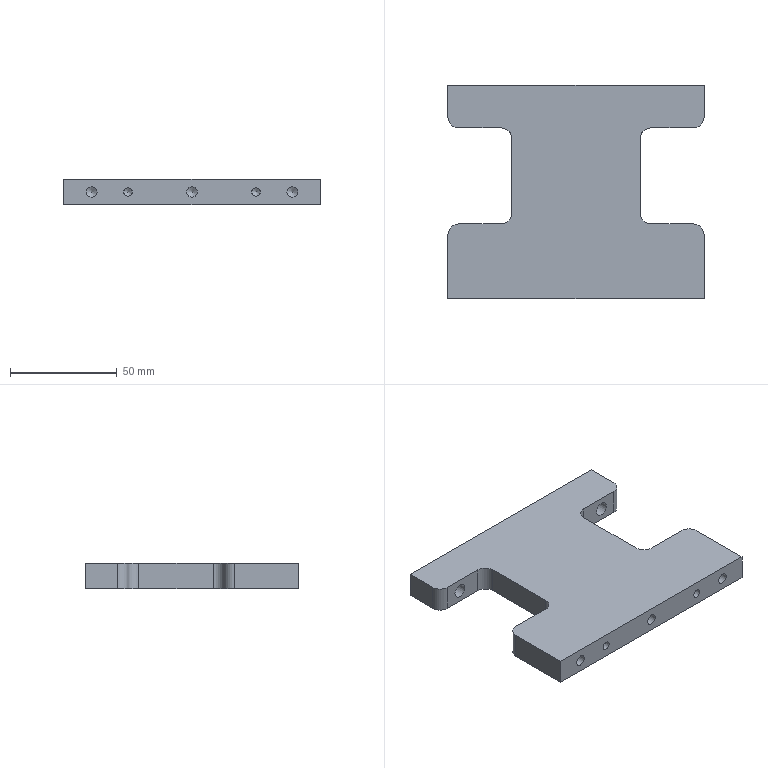Part | STEP file | SynoNew-0304-024 | 1 solid | 34 faces | box 120 x 100 x 12 mm | volume 109561 mm3 | cylinder 15 | plane 14 | cone 5 | commonest cylinder face diameters 10 x8 5 x3 4 x2 6.5 x2
STEP:
#1=CARTESIAN_POINT('',(32.,-42.,6.));
#2=VERTEX_POINT('',#1);
#3=CARTESIAN_POINT('',(28.,-42.,6.));
#4=VERTEX_POINT('',#3);
#5=CARTESIAN_POINT('',(30.,-42.,6.));
#6=DIRECTION('',(0.,-1.,0.));
#7=DIRECTION('',(1.,0.,0.));
#8=AXIS2_PLACEMENT_3D('',#5,#6,#7);
#9=CIRCLE('',#8,2.);
#10=EDGE_CURVE('',#2,#4,#9,.T.);
#11=ORIENTED_EDGE('',*,*,#10,.T.);
#12=CARTESIAN_POINT('',(30.,-40.798,6.));
#13=VERTEX_POINT('',#12);
#14=CARTESIAN_POINT('',(29.,-41.399,6.));
#15=DIRECTION('',(0.8572,0.515,0.));
#16=VECTOR('',#15,1.);
#17=LINE('',#14,#16);
#18=EDGE_CURVE('',#4,#13,#17,.T.);
#19=ORIENTED_EDGE('',*,*,#18,.T.);
#20=ORIENTED_EDGE('',*,*,#18,.F.);
#21=CARTESIAN_POINT('',(30.,-42.,6.));
#22=DIRECTION('',(0.,-1.,0.));
#23=DIRECTION('',(1.,0.,0.));
#24=AXIS2_PLACEMENT_3D('',#21,#22,#23);
#25=CIRCLE('',#24,2.);
#26=EDGE_CURVE('',#4,#2,#25,.T.);
#27=ORIENTED_EDGE('',*,*,#26,.T.);
#28=EDGE_LOOP('',(#11,#19,#20,#27));
#29=FACE_OUTER_BOUND('',#28,.T.);
#30=CARTESIAN_POINT('',(30.,-41.399,6.));
#31=DIRECTION('',(0.,-1.,0.));
#32=DIRECTION('',(1.,0.,0.));
#33=AXIS2_PLACEMENT_3D('',#30,#31,#32);
#34=CONICAL_SURFACE('',#33,1.,1.03);
#35=ADVANCED_FACE('',(#29),#34,.F.);
#36=CARTESIAN_POINT('',(32.,-50.,6.));
#37=VERTEX_POINT('',#36);
#38=CARTESIAN_POINT('',(28.,-50.,6.));
#39=VERTEX_POINT('',#38);
#40=CARTESIAN_POINT('',(30.,-50.,6.));
#41=DIRECTION('',(0.,1.,0.));
#42=DIRECTION('',(1.,0.,0.));
#43=AXIS2_PLACEMENT_3D('',#40,#41,#42);
#44=CIRCLE('',#43,2.);
#45=EDGE_CURVE('',#37,#39,#44,.T.);
#46=ORIENTED_EDGE('',*,*,#45,.F.);
#47=CARTESIAN_POINT('',(30.,-50.,6.));
#48=DIRECTION('',(0.,1.,0.));
#49=DIRECTION('',(1.,0.,0.));
#50=AXIS2_PLACEMENT_3D('',#47,#48,#49);
#51=CIRCLE('',#50,2.);
#52=EDGE_CURVE('',#39,#37,#51,.T.);
#53=ORIENTED_EDGE('',*,*,#52,.F.);
#54=CARTESIAN_POINT('',(28.,-46.,6.));
#55=DIRECTION('',(0.,1.,0.));
#56=VECTOR('',#55,2.);
#57=LINE('',#54,#56);
#58=EDGE_CURVE('',#39,#4,#57,.T.);
#59=ORIENTED_EDGE('',*,*,#58,.T.);
#60=ORIENTED_EDGE('',*,*,#10,.F.);
#61=ORIENTED_EDGE('',*,*,#26,.F.);
#62=ORIENTED_EDGE('',*,*,#58,.F.);
#63=EDGE_LOOP('',(#46,#53,#59,#60,#61,#62));
#64=FACE_OUTER_BOUND('',#63,.T.);
#65=CARTESIAN_POINT('',(30.,-46.,6.));
#66=DIRECTION('',(0.,-1.,0.));
#67=DIRECTION('',(1.,0.,0.));
#68=AXIS2_PLACEMENT_3D('',#65,#66,#67);
#69=CYLINDRICAL_SURFACE('',#68,2.);
#70=ADVANCED_FACE('',(#64),#69,.F.);
#71=CARTESIAN_POINT('',(-28.,-42.,6.));
#72=VERTEX_POINT('',#71);
#73=CARTESIAN_POINT('',(-32.,-42.,6.));
#74=VERTEX_POINT('',#73);
#75=CARTESIAN_POINT('',(-30.,-42.,6.));
#76=DIRECTION('',(0.,-1.,0.));
#77=DIRECTION('',(1.,0.,0.));
#78=AXIS2_PLACEMENT_3D('',#75,#76,#77);
#79=CIRCLE('',#78,2.);
#80=EDGE_CURVE('',#72,#74,#79,.T.);
#81=ORIENTED_EDGE('',*,*,#80,.T.);
#82=CARTESIAN_POINT('',(-30.,-40.798,6.));
#83=VERTEX_POINT('',#82);
#84=CARTESIAN_POINT('',(-31.,-41.399,6.));
#85=DIRECTION('',(0.8572,0.515,0.));
#86=VECTOR('',#85,1.);
#87=LINE('',#84,#86);
#88=EDGE_CURVE('',#74,#83,#87,.T.);
#89=ORIENTED_EDGE('',*,*,#88,.T.);
#90=ORIENTED_EDGE('',*,*,#88,.F.);
#91=CARTESIAN_POINT('',(-30.,-42.,6.));
#92=DIRECTION('',(0.,-1.,0.));
#93=DIRECTION('',(1.,0.,0.));
#94=AXIS2_PLACEMENT_3D('',#91,#92,#93);
#95=CIRCLE('',#94,2.);
#96=EDGE_CURVE('',#74,#72,#95,.T.);
#97=ORIENTED_EDGE('',*,*,#96,.T.);
#98=EDGE_LOOP('',(#81,#89,#90,#97));
#99=FACE_OUTER_BOUND('',#98,.T.);
#100=CARTESIAN_POINT('',(-30.,-41.399,6.));
#101=DIRECTION('',(0.,-1.,0.));
#102=DIRECTION('',(1.,0.,0.));
#103=AXIS2_PLACEMENT_3D('',#100,#101,#102);
#104=CONICAL_SURFACE('',#103,1.,1.03);
#105=ADVANCED_FACE('',(#99),#104,.F.);
#106=CARTESIAN_POINT('',(-28.,-50.,6.));
#107=VERTEX_POINT('',#106);
#108=CARTESIAN_POINT('',(-32.,-50.,6.));
#109=VERTEX_POINT('',#108);
#110=CARTESIAN_POINT('',(-30.,-50.,6.));
#111=DIRECTION('',(0.,1.,0.));
#112=DIRECTION('',(1.,0.,0.));
#113=AXIS2_PLACEMENT_3D('',#110,#111,#112);
#114=CIRCLE('',#113,2.);
#115=EDGE_CURVE('',#107,#109,#114,.T.);
#116=ORIENTED_EDGE('',*,*,#115,.F.);
#117=CARTESIAN_POINT('',(-30.,-50.,6.));
#118=DIRECTION('',(0.,1.,0.));
#119=DIRECTION('',(1.,0.,0.));
#120=AXIS2_PLACEMENT_3D('',#117,#118,#119);
#121=CIRCLE('',#120,2.);
#122=EDGE_CURVE('',#109,#107,#121,.T.);
#123=ORIENTED_EDGE('',*,*,#122,.F.);
#124=CARTESIAN_POINT('',(-32.,-46.,6.));
#125=DIRECTION('',(0.,1.,0.));
#126=VECTOR('',#125,2.);
#127=LINE('',#124,#126);
#128=EDGE_CURVE('',#109,#74,#127,.T.);
#129=ORIENTED_EDGE('',*,*,#128,.T.);
#130=ORIENTED_EDGE('',*,*,#80,.F.);
#131=ORIENTED_EDGE('',*,*,#96,.F.);
#132=ORIENTED_EDGE('',*,*,#128,.F.);
#133=EDGE_LOOP('',(#116,#123,#129,#130,#131,#132));
#134=FACE_OUTER_BOUND('',#133,.T.);
#135=CARTESIAN_POINT('',(-30.,-46.,6.));
#136=DIRECTION('',(0.,-1.,0.));
#137=DIRECTION('',(1.,0.,0.));
#138=AXIS2_PLACEMENT_3D('',#135,#136,#137);
#139=CYLINDRICAL_SURFACE('',#138,2.);
#140=ADVANCED_FACE('',(#134),#139,.F.);
#141=CARTESIAN_POINT('',(2.5,-42.,6.));
#142=VERTEX_POINT('',#141);
#143=CARTESIAN_POINT('',(-2.5,-42.,6.));
#144=VERTEX_POINT('',#143);
#145=CARTESIAN_POINT('',(0.,-42.,6.));
#146=DIRECTION('',(0.,-1.,0.));
#147=DIRECTION('',(1.,0.,0.));
#148=AXIS2_PLACEMENT_3D('',#145,#146,#147);
#149=CIRCLE('',#148,2.5);
#150=EDGE_CURVE('',#142,#144,#149,.T.);
#151=ORIENTED_EDGE('',*,*,#150,.T.);
#152=CARTESIAN_POINT('',(0.,-40.498,6.));
#153=VERTEX_POINT('',#152);
#154=CARTESIAN_POINT('',(-1.25,-41.249,6.));
#155=DIRECTION('',(0.8572,0.515,0.));
#156=VECTOR('',#155,1.25);
#157=LINE('',#154,#156);
#158=EDGE_CURVE('',#144,#153,#157,.T.);
#159=ORIENTED_EDGE('',*,*,#158,.T.);
#160=ORIENTED_EDGE('',*,*,#158,.F.);
#161=CARTESIAN_POINT('',(0.,-42.,6.));
#162=DIRECTION('',(0.,-1.,0.));
#163=DIRECTION('',(1.,0.,0.));
#164=AXIS2_PLACEMENT_3D('',#161,#162,#163);
#165=CIRCLE('',#164,2.5);
#166=EDGE_CURVE('',#144,#142,#165,.T.);
#167=ORIENTED_EDGE('',*,*,#166,.T.);
#168=EDGE_LOOP('',(#151,#159,#160,#167));
#169=FACE_OUTER_BOUND('',#168,.T.);
#170=CARTESIAN_POINT('',(0.,-41.249,6.));
#171=DIRECTION('',(0.,-1.,0.));
#172=DIRECTION('',(1.,0.,0.));
#173=AXIS2_PLACEMENT_3D('',#170,#171,#172);
#174=CONICAL_SURFACE('',#173,1.25,1.03);
#175=ADVANCED_FACE('',(#169),#174,.F.);
#176=CARTESIAN_POINT('',(2.5,-50.,6.));
#177=VERTEX_POINT('',#176);
#178=CARTESIAN_POINT('',(-2.5,-50.,6.));
#179=VERTEX_POINT('',#178);
#180=CARTESIAN_POINT('',(0.,-50.,6.));
#181=DIRECTION('',(0.,1.,0.));
#182=DIRECTION('',(1.,0.,0.));
#183=AXIS2_PLACEMENT_3D('',#180,#181,#182);
#184=CIRCLE('',#183,2.5);
#185=EDGE_CURVE('',#177,#179,#184,.T.);
#186=ORIENTED_EDGE('',*,*,#185,.F.);
#187=CARTESIAN_POINT('',(0.,-50.,6.));
#188=DIRECTION('',(0.,1.,0.));
#189=DIRECTION('',(1.,0.,0.));
#190=AXIS2_PLACEMENT_3D('',#187,#188,#189);
#191=CIRCLE('',#190,2.5);
#192=EDGE_CURVE('',#179,#177,#191,.T.);
#193=ORIENTED_EDGE('',*,*,#192,.F.);
#194=CARTESIAN_POINT('',(-2.5,-46.,6.));
#195=DIRECTION('',(0.,1.,0.));
#196=VECTOR('',#195,2.5);
#197=LINE('',#194,#196);
#198=EDGE_CURVE('',#179,#144,#197,.T.);
#199=ORIENTED_EDGE('',*,*,#198,.T.);
#200=ORIENTED_EDGE('',*,*,#150,.F.);
#201=ORIENTED_EDGE('',*,*,#166,.F.);
#202=ORIENTED_EDGE('',*,*,#198,.F.);
#203=EDGE_LOOP('',(#186,#193,#199,#200,#201,#202));
#204=FACE_OUTER_BOUND('',#203,.T.);
#205=CARTESIAN_POINT('',(0.,-46.,6.));
#206=DIRECTION('',(0.,-1.,0.));
#207=DIRECTION('',(1.,0.,0.));
#208=AXIS2_PLACEMENT_3D('',#205,#206,#207);
#209=CYLINDRICAL_SURFACE('',#208,2.5);
#210=ADVANCED_FACE('',(#204),#209,.F.);
#211=CARTESIAN_POINT('',(49.5,-42.,6.));
#212=VERTEX_POINT('',#211);
#213=CARTESIAN_POINT('',(44.5,-42.,6.));
#214=VERTEX_POINT('',#213);
#215=CARTESIAN_POINT('',(47.,-42.,6.));
#216=DIRECTION('',(0.,-1.,0.));
#217=DIRECTION('',(1.,0.,0.));
#218=AXIS2_PLACEMENT_3D('',#215,#216,#217);
#219=CIRCLE('',#218,2.5);
#220=EDGE_CURVE('',#212,#214,#219,.T.);
#221=ORIENTED_EDGE('',*,*,#220,.T.);
#222=CARTESIAN_POINT('',(47.,-40.498,6.));
#223=VERTEX_POINT('',#222);
#224=CARTESIAN_POINT('',(45.75,-41.249,6.));
#225=DIRECTION('',(0.8572,0.515,0.));
#226=VECTOR('',#225,1.25);
#227=LINE('',#224,#226);
#228=EDGE_CURVE('',#214,#223,#227,.T.);
#229=ORIENTED_EDGE('',*,*,#228,.T.);
#230=ORIENTED_EDGE('',*,*,#228,.F.);
#231=CARTESIAN_POINT('',(47.,-42.,6.));
#232=DIRECTION('',(0.,-1.,0.));
#233=DIRECTION('',(1.,0.,0.));
#234=AXIS2_PLACEMENT_3D('',#231,#232,#233);
#235=CIRCLE('',#234,2.5);
#236=EDGE_CURVE('',#214,#212,#235,.T.);
#237=ORIENTED_EDGE('',*,*,#236,.T.);
#238=EDGE_LOOP('',(#221,#229,#230,#237));
#239=FACE_OUTER_BOUND('',#238,.T.);
#240=CARTESIAN_POINT('',(47.,-41.249,6.));
#241=DIRECTION('',(0.,-1.,0.));
#242=DIRECTION('',(1.,0.,0.));
#243=AXIS2_PLACEMENT_3D('',#240,#241,#242);
#244=CONICAL_SURFACE('',#243,1.25,1.03);
#245=ADVANCED_FACE('',(#239),#244,.F.);
#246=CARTESIAN_POINT('',(49.5,-50.,6.));
#247=VERTEX_POINT('',#246);
#248=CARTESIAN_POINT('',(44.5,-50.,6.));
#249=VERTEX_POINT('',#248);
#250=CARTESIAN_POINT('',(47.,-50.,6.));
#251=DIRECTION('',(0.,1.,0.));
#252=DIRECTION('',(1.,0.,0.));
#253=AXIS2_PLACEMENT_3D('',#250,#251,#252);
#254=CIRCLE('',#253,2.5);
#255=EDGE_CURVE('',#247,#249,#254,.T.);
#256=ORIENTED_EDGE('',*,*,#255,.F.);
#257=CARTESIAN_POINT('',(47.,-50.,6.));
#258=DIRECTION('',(0.,1.,0.));
#259=DIRECTION('',(1.,0.,0.));
#260=AXIS2_PLACEMENT_3D('',#257,#258,#259);
#261=CIRCLE('',#260,2.5);
#262=EDGE_CURVE('',#249,#247,#261,.T.);
#263=ORIENTED_EDGE('',*,*,#262,.F.);
#264=CARTESIAN_POINT('',(44.5,-46.,6.));
#265=DIRECTION('',(0.,1.,0.));
#266=VECTOR('',#265,2.5);
#267=LINE('',#264,#266);
#268=EDGE_CURVE('',#249,#214,#267,.T.);
#269=ORIENTED_EDGE('',*,*,#268,.T.);
#270=ORIENTED_EDGE('',*,*,#220,.F.);
#271=ORIENTED_EDGE('',*,*,#236,.F.);
#272=ORIENTED_EDGE('',*,*,#268,.F.);
#273=EDGE_LOOP('',(#256,#263,#269,#270,#271,#272));
#274=FACE_OUTER_BOUND('',#273,.T.);
#275=CARTESIAN_POINT('',(47.,-46.,6.));
#276=DIRECTION('',(0.,-1.,0.));
#277=DIRECTION('',(1.,0.,0.));
#278=AXIS2_PLACEMENT_3D('',#275,#276,#277);
#279=CYLINDRICAL_SURFACE('',#278,2.5);
#280=ADVANCED_FACE('',(#274),#279,.F.);
#281=CARTESIAN_POINT('',(-44.5,-42.,6.));
#282=VERTEX_POINT('',#281);
#283=CARTESIAN_POINT('',(-49.5,-42.,6.));
#284=VERTEX_POINT('',#283);
#285=CARTESIAN_POINT('',(-47.,-42.,6.));
#286=DIRECTION('',(0.,-1.,0.));
#287=DIRECTION('',(1.,0.,0.));
#288=AXIS2_PLACEMENT_3D('',#285,#286,#287);
#289=CIRCLE('',#288,2.5);
#290=EDGE_CURVE('',#282,#284,#289,.T.);
#291=ORIENTED_EDGE('',*,*,#290,.T.);
#292=CARTESIAN_POINT('',(-47.,-40.498,6.));
#293=VERTEX_POINT('',#292);
#294=CARTESIAN_POINT('',(-48.25,-41.249,6.));
#295=DIRECTION('',(0.8572,0.515,0.));
#296=VECTOR('',#295,1.25);
#297=LINE('',#294,#296);
#298=EDGE_CURVE('',#284,#293,#297,.T.);
#299=ORIENTED_EDGE('',*,*,#298,.T.);
#300=ORIENTED_EDGE('',*,*,#298,.F.);
#301=CARTESIAN_POINT('',(-47.,-42.,6.));
#302=DIRECTION('',(0.,-1.,0.));
#303=DIRECTION('',(1.,0.,0.));
#304=AXIS2_PLACEMENT_3D('',#301,#302,#303);
#305=CIRCLE('',#304,2.5);
#306=EDGE_CURVE('',#284,#282,#305,.T.);
#307=ORIENTED_EDGE('',*,*,#306,.T.);
#308=EDGE_LOOP('',(#291,#299,#300,#307));
#309=FACE_OUTER_BOUND('',#308,.T.);
#310=CARTESIAN_POINT('',(-47.,-41.249,6.));
#311=DIRECTION('',(0.,-1.,0.));
#312=DIRECTION('',(1.,0.,0.));
#313=AXIS2_PLACEMENT_3D('',#310,#311,#312);
#314=CONICAL_SURFACE('',#313,1.25,1.03);
#315=ADVANCED_FACE('',(#309),#314,.F.);
#316=CARTESIAN_POINT('',(-44.5,-50.,6.));
#317=VERTEX_POINT('',#316);
#318=CARTESIAN_POINT('',(-49.5,-50.,6.));
#319=VERTEX_POINT('',#318);
#320=CARTESIAN_POINT('',(-47.,-50.,6.));
#321=DIRECTION('',(0.,1.,0.));
#322=DIRECTION('',(1.,0.,0.));
#323=AXIS2_PLACEMENT_3D('',#320,#321,#322);
#324=CIRCLE('',#323,2.5);
#325=EDGE_CURVE('',#317,#319,#324,.T.);
#326=ORIENTED_EDGE('',*,*,#325,.F.);
#327=CARTESIAN_POINT('',(-47.,-50.,6.));
#328=DIRECTION('',(0.,1.,0.));
#329=DIRECTION('',(1.,0.,0.));
#330=AXIS2_PLACEMENT_3D('',#327,#328,#329);
#331=CIRCLE('',#330,2.5);
#332=EDGE_CURVE('',#319,#317,#331,.T.);
#333=ORIENTED_EDGE('',*,*,#332,.F.);
#334=CARTESIAN_POINT('',(-49.5,-46.,6.));
#335=DIRECTION('',(0.,1.,0.));
#336=VECTOR('',#335,2.5);
#337=LINE('',#334,#336);
#338=EDGE_CURVE('',#319,#284,#337,.T.);
#339=ORIENTED_EDGE('',*,*,#338,.T.);
#340=ORIENTED_EDGE('',*,*,#290,.F.);
#341=ORIENTED_EDGE('',*,*,#306,.F.);
#342=ORIENTED_EDGE('',*,*,#338,.F.);
#343=EDGE_LOOP('',(#326,#333,#339,#340,#341,#342));
#344=FACE_OUTER_BOUND('',#343,.T.);
#345=CARTESIAN_POINT('',(-47.,-46.,6.));
#346=DIRECTION('',(0.,-1.,0.));
#347=DIRECTION('',(1.,0.,0.));
#348=AXIS2_PLACEMENT_3D('',#345,#346,#347);
#349=CYLINDRICAL_SURFACE('',#348,2.5);
#350=ADVANCED_FACE('',(#344),#349,.F.);
#351=CARTESIAN_POINT('',(55.,-15.,12.));
#352=VERTEX_POINT('',#351);
#353=CARTESIAN_POINT('',(60.,-20.,12.));
#354=VERTEX_POINT('',#353);
#355=CARTESIAN_POINT('',(55.,-20.,12.));
#356=DIRECTION('',(0.,0.,-1.));
#357=DIRECTION('',(0.7071,0.7071,0.));
#358=AXIS2_PLACEMENT_3D('',#355,#356,#357);
#359=CIRCLE('',#358,5.);
#360=EDGE_CURVE('',#352,#354,#359,.T.);
#361=ORIENTED_EDGE('',*,*,#360,.T.);
#362=CARTESIAN_POINT('',(60.,-20.,0.));
#363=VERTEX_POINT('',#362);
#364=CARTESIAN_POINT('',(60.,-20.,6.));
#365=DIRECTION('',(0.,0.,-1.));
#366=VECTOR('',#365,10.);
#367=LINE('',#364,#366);
#368=EDGE_CURVE('',#354,#363,#367,.T.);
#369=ORIENTED_EDGE('',*,*,#368,.T.);
#370=CARTESIAN_POINT('',(55.,-15.,0.));
#371=VERTEX_POINT('',#370);
#372=CARTESIAN_POINT('',(55.,-20.,0.));
#373=DIRECTION('',(0.,0.,1.));
#374=DIRECTION('',(0.7071,0.7071,0.));
#375=AXIS2_PLACEMENT_3D('',#372,#373,#374);
#376=CIRCLE('',#375,5.);
#377=EDGE_CURVE('',#363,#371,#376,.T.);
#378=ORIENTED_EDGE('',*,*,#377,.T.);
#379=CARTESIAN_POINT('',(55.,-15.,6.));
#380=DIRECTION('',(0.,0.,1.));
#381=VECTOR('',#380,10.);
#382=LINE('',#379,#381);
#383=EDGE_CURVE('',#371,#352,#382,.T.);
#384=ORIENTED_EDGE('',*,*,#383,.T.);
#385=EDGE_LOOP('',(#361,#369,#378,#384));
#386=FACE_OUTER_BOUND('',#385,.T.);
#387=CARTESIAN_POINT('',(55.,-20.,6.));
#388=DIRECTION('',(0.,0.,1.));
#389=DIRECTION('',(0.7071,0.7071,0.));
#390=AXIS2_PLACEMENT_3D('',#387,#388,#389);
#391=CYLINDRICAL_SURFACE('',#390,5.);
#392=ADVANCED_FACE('',(#386),#391,.T.);
#393=ORIENTED_EDGE('',*,*,#368,.F.);
#394=CARTESIAN_POINT('',(60.,-50.,12.));
#395=VERTEX_POINT('',#394);
#396=CARTESIAN_POINT('',(60.,-50.,12.));
#397=DIRECTION('',(0.,1.,0.));
#398=VECTOR('',#397,10.);
#399=LINE('',#396,#398);
#400=EDGE_CURVE('',#395,#354,#399,.T.);
#401=ORIENTED_EDGE('',*,*,#400,.F.);
#402=CARTESIAN_POINT('',(60.,-50.,0.));
#403=VERTEX_POINT('',#402);
#404=CARTESIAN_POINT('',(60.,-50.,0.));
#405=DIRECTION('',(0.,0.,1.));
#406=VECTOR('',#405,10.);
#407=LINE('',#404,#406);
#408=EDGE_CURVE('',#403,#395,#407,.T.);
#409=ORIENTED_EDGE('',*,*,#408,.F.);
#410=CARTESIAN_POINT('',(60.,-50.,0.));
#411=DIRECTION('',(0.,1.,0.));
#412=VECTOR('',#411,10.);
#413=LINE('',#410,#412);
#414=EDGE_CURVE('',#403,#363,#413,.T.);
#415=ORIENTED_EDGE('',*,*,#414,.T.);
#416=EDGE_LOOP('',(#393,#401,#409,#415));
#417=FACE_OUTER_BOUND('',#416,.T.);
#418=CARTESIAN_POINT('',(60.,-50.,0.));
#419=DIRECTION('',(1.,0.,0.));
#420=DIRECTION('',(0.,1.,0.));
#421=AXIS2_PLACEMENT_3D('',#418,#419,#420);
#422=PLANE('',#421);
#423=ADVANCED_FACE('',(#417),#422,.T.);
#424=ORIENTED_EDGE('',*,*,#360,.F.);
#425=CARTESIAN_POINT('',(35.,-15.,12.));
#426=VERTEX_POINT('',#425);
#427=CARTESIAN_POINT('',(39.479,-15.,12.));
#428=DIRECTION('',(-1.,0.,0.));
#429=VECTOR('',#428,10.);
#430=LINE('',#427,#429);
#431=EDGE_CURVE('',#352,#426,#430,.T.);
#432=ORIENTED_EDGE('',*,*,#431,.T.);
#433=CARTESIAN_POINT('',(30.,-10.,12.));
#434=VERTEX_POINT('',#433);
#435=CARTESIAN_POINT('',(35.,-10.,12.));
#436=DIRECTION('',(0.,0.,1.));
#437=DIRECTION('',(-0.7071,-0.7071,0.));
#438=AXIS2_PLACEMENT_3D('',#435,#436,#437);
#439=CIRCLE('',#438,5.);
#440=EDGE_CURVE('',#434,#426,#439,.T.);
#441=ORIENTED_EDGE('',*,*,#440,.F.);
#442=CARTESIAN_POINT('',(30.,25.,12.));
#443=VERTEX_POINT('',#442);
#444=CARTESIAN_POINT('',(30.,-7.5,12.));
#445=DIRECTION('',(0.,1.,0.));
#446=VECTOR('',#445,10.);
#447=LINE('',#444,#446);
#448=EDGE_CURVE('',#434,#443,#447,.T.);
#449=ORIENTED_EDGE('',*,*,#448,.T.);
#450=CARTESIAN_POINT('',(35.,30.,12.));
#451=VERTEX_POINT('',#450);
#452=CARTESIAN_POINT('',(35.,25.,12.));
#453=DIRECTION('',(0.,0.,1.));
#454=DIRECTION('',(-0.7071,0.7071,0.));
#455=AXIS2_PLACEMENT_3D('',#452,#453,#454);
#456=CIRCLE('',#455,5.);
#457=EDGE_CURVE('',#451,#443,#456,.T.);
#458=ORIENTED_EDGE('',*,*,#457,.F.);
#459=CARTESIAN_POINT('',(55.,30.,12.));
#460=VERTEX_POINT('',#459);
#461=CARTESIAN_POINT('',(15.,30.,12.));
#462=DIRECTION('',(1.,0.,0.));
#463=VECTOR('',#462,10.);
#464=LINE('',#461,#463);
#465=EDGE_CURVE('',#451,#460,#464,.T.);
#466=ORIENTED_EDGE('',*,*,#465,.T.);
#467=CARTESIAN_POINT('',(60.,35.,12.));
#468=VERTEX_POINT('',#467);
#469=CARTESIAN_POINT('',(55.,35.,12.));
#470=DIRECTION('',(0.,0.,-1.));
#471=DIRECTION('',(0.7071,-0.7071,0.));
#472=AXIS2_PLACEMENT_3D('',#469,#470,#471);
#473=CIRCLE('',#472,5.);
#474=EDGE_CURVE('',#468,#460,#473,.T.);
#475=ORIENTED_EDGE('',*,*,#474,.F.);
#476=CARTESIAN_POINT('',(60.,50.,12.));
#477=VERTEX_POINT('',#476);
#478=CARTESIAN_POINT('',(60.,-50.,12.));
#479=DIRECTION('',(0.,1.,0.));
#480=VECTOR('',#479,10.);
#481=LINE('',#478,#480);
#482=EDGE_CURVE('',#468,#477,#481,.T.);
#483=ORIENTED_EDGE('',*,*,#482,.T.);
#484=CARTESIAN_POINT('',(-60.,50.,12.));
#485=VERTEX_POINT('',#484);
#486=CARTESIAN_POINT('',(60.,50.,12.));
#487=DIRECTION('',(-1.,0.,0.));
#488=VECTOR('',#487,10.);
#489=LINE('',#486,#488);
#490=EDGE_CURVE('',#477,#485,#489,.T.);
#491=ORIENTED_EDGE('',*,*,#490,.T.);
#492=CARTESIAN_POINT('',(-60.,35.,12.));
#493=VERTEX_POINT('',#492);
#494=CARTESIAN_POINT('',(-60.,50.,12.));
#495=DIRECTION('',(0.,-1.,0.));
#496=VECTOR('',#495,10.);
#497=LINE('',#494,#496);
#498=EDGE_CURVE('',#485,#493,#497,.T.);
#499=ORIENTED_EDGE('',*,*,#498,.T.);
#500=CARTESIAN_POINT('',(-55.,30.,12.));
#501=VERTEX_POINT('',#500);
#502=CARTESIAN_POINT('',(-55.,35.,12.));
#503=DIRECTION('',(0.,0.,-1.));
#504=DIRECTION('',(-0.7071,-0.7071,0.));
#505=AXIS2_PLACEMENT_3D('',#502,#503,#504);
#506=CIRCLE('',#505,5.);
#507=EDGE_CURVE('',#501,#493,#506,.T.);
#508=ORIENTED_EDGE('',*,*,#507,.F.);
#509=CARTESIAN_POINT('',(-35.,30.,12.));
#510=VERTEX_POINT('',#509);
#511=CARTESIAN_POINT('',(-15.,30.,12.));
#512=DIRECTION('',(1.,0.,0.));
#513=VECTOR('',#512,10.);
#514=LINE('',#511,#513);
#515=EDGE_CURVE('',#501,#510,#514,.T.);
#516=ORIENTED_EDGE('',*,*,#515,.T.);
#517=CARTESIAN_POINT('',(-30.,25.,12.));
#518=VERTEX_POINT('',#517);
#519=CARTESIAN_POINT('',(-35.,25.,12.));
#520=DIRECTION('',(0.,0.,1.));
#521=DIRECTION('',(0.7071,0.7071,0.));
#522=AXIS2_PLACEMENT_3D('',#519,#520,#521);
#523=CIRCLE('',#522,5.);
#524=EDGE_CURVE('',#518,#510,#523,.T.);
#525=ORIENTED_EDGE('',*,*,#524,.F.);
#526=CARTESIAN_POINT('',(-30.,-10.,12.));
#527=VERTEX_POINT('',#526);
#528=CARTESIAN_POINT('',(-30.,-7.5,12.));
#529=DIRECTION('',(0.,-1.,0.));
#530=VECTOR('',#529,10.);
#531=LINE('',#528,#530);
#532=EDGE_CURVE('',#518,#527,#531,.T.);
#533=ORIENTED_EDGE('',*,*,#532,.T.);
#534=CARTESIAN_POINT('',(-35.,-15.,12.));
#535=VERTEX_POINT('',#534);
#536=CARTESIAN_POINT('',(-35.,-10.,12.));
#537=DIRECTION('',(0.,0.,1.));
#538=DIRECTION('',(0.7071,-0.7071,0.));
#539=AXIS2_PLACEMENT_3D('',#536,#537,#538);
#540=CIRCLE('',#539,5.);
#541=EDGE_CURVE('',#535,#527,#540,.T.);
#542=ORIENTED_EDGE('',*,*,#541,.F.);
#543=CARTESIAN_POINT('',(-55.,-15.,12.));
#544=VERTEX_POINT('',#543);
#545=CARTESIAN_POINT('',(-39.479,-15.,12.));
#546=DIRECTION('',(-1.,0.,0.));
#547=VECTOR('',#546,10.);
#548=LINE('',#545,#547);
#549=EDGE_CURVE('',#535,#544,#548,.T.);
#550=ORIENTED_EDGE('',*,*,#549,.T.);
#551=CARTESIAN_POINT('',(-60.,-20.,12.));
#552=VERTEX_POINT('',#551);
#553=CARTESIAN_POINT('',(-55.,-20.,12.));
#554=DIRECTION('',(0.,0.,-1.));
#555=DIRECTION('',(-0.7071,0.7071,0.));
#556=AXIS2_PLACEMENT_3D('',#553,#554,#555);
#557=CIRCLE('',#556,5.);
#558=EDGE_CURVE('',#552,#544,#557,.T.);
#559=ORIENTED_EDGE('',*,*,#558,.F.);
#560=CARTESIAN_POINT('',(-60.,-50.,12.));
#561=VERTEX_POINT('',#560);
#562=CARTESIAN_POINT('',(-60.,50.,12.));
#563=DIRECTION('',(0.,-1.,0.));
#564=VECTOR('',#563,10.);
#565=LINE('',#562,#564);
#566=EDGE_CURVE('',#552,#561,#565,.T.);
#567=ORIENTED_EDGE('',*,*,#566,.T.);
#568=CARTESIAN_POINT('',(-60.,-50.,12.));
#569=DIRECTION('',(1.,0.,0.));
#570=VECTOR('',#569,10.);
#571=LINE('',#568,#570);
#572=EDGE_CURVE('',#561,#395,#571,.T.);
#573=ORIENTED_EDGE('',*,*,#572,.T.);
#574=ORIENTED_EDGE('',*,*,#400,.T.);
#575=EDGE_LOOP('',(#424,#432,#441,#449,#458,#466,#475,#483,#491,#499,#508,#516,#525,#533,#542,#550,#559,#567,#573,#574));
#576=FACE_OUTER_BOUND('',#575,.T.);
#577=CARTESIAN_POINT('',(0.,0.,12.));
#578=DIRECTION('',(0.,0.,1.));
#579=DIRECTION('',(1.,0.,0.));
#580=AXIS2_PLACEMENT_3D('',#577,#578,#579);
#581=PLANE('',#580);
#582=ADVANCED_FACE('',(#576),#581,.T.);
#583=CARTESIAN_POINT('',(-55.,-15.,0.));
#584=VERTEX_POINT('',#583);
#585=CARTESIAN_POINT('',(-60.,-20.,0.));
#586=VERTEX_POINT('',#585);
#587=CARTESIAN_POINT('',(-55.,-20.,0.));
#588=DIRECTION('',(0.,0.,1.));
#589=DIRECTION('',(-0.7071,0.7071,0.));
#590=AXIS2_PLACEMENT_3D('',#587,#588,#589);
#591=CIRCLE('',#590,5.);
#592=EDGE_CURVE('',#584,#586,#591,.T.);
#593=ORIENTED_EDGE('',*,*,#592,.T.);
#594=CARTESIAN_POINT('',(-60.,-20.,6.));
#595=DIRECTION('',(0.,0.,1.));
#596=VECTOR('',#595,10.);
#597=LINE('',#594,#596);
#598=EDGE_CURVE('',#586,#552,#597,.T.);
#599=ORIENTED_EDGE('',*,*,#598,.T.);
#600=ORIENTED_EDGE('',*,*,#558,.T.);
#601=CARTESIAN_POINT('',(-55.,-15.,6.));
#602=DIRECTION('',(0.,0.,-1.));
#603=VECTOR('',#602,10.);
#604=LINE('',#601,#603);
#605=EDGE_CURVE('',#544,#584,#604,.T.);
#606=ORIENTED_EDGE('',*,*,#605,.T.);
#607=EDGE_LOOP('',(#593,#599,#600,#606));
#608=FACE_OUTER_BOUND('',#607,.T.);
#609=CARTESIAN_POINT('',(-55.,-20.,6.));
#610=DIRECTION('',(0.,0.,-1.));
#611=DIRECTION('',(-0.7071,0.7071,0.));
#612=AXIS2_PLACEMENT_3D('',#609,#610,#611);
#613=CYLINDRICAL_SURFACE('',#612,5.);
#614=ADVANCED_FACE('',(#608),#613,.T.);
#615=ORIENTED_EDGE('',*,*,#605,.F.);
#616=ORIENTED_EDGE('',*,*,#549,.F.);
#617=CARTESIAN_POINT('',(-35.,-15.,0.));
#618=VERTEX_POINT('',#617);
#619=CARTESIAN_POINT('',(-35.,-15.,12.));
#620=DIRECTION('',(0.,0.,1.));
#621=VECTOR('',#620,10.);
#622=LINE('',#619,#621);
#623=EDGE_CURVE('',#618,#535,#622,.T.);
#624=ORIENTED_EDGE('',*,*,#623,.F.);
#625=CARTESIAN_POINT('',(-39.479,-15.,0.));
#626=DIRECTION('',(1.,0.,0.));
#627=VECTOR('',#626,10.);
#628=LINE('',#625,#627);
#629=EDGE_CURVE('',#584,#618,#628,.T.);
#630=ORIENTED_EDGE('',*,*,#629,.F.);
#631=EDGE_LOOP('',(#615,#616,#624,#630));
#632=FACE_OUTER_BOUND('',#631,.T.);
#633=CARTESIAN_POINT('',(-78.957,-15.,12.));
#634=DIRECTION('',(0.,1.,0.));
#635=DIRECTION('',(1.,0.,0.));
#636=AXIS2_PLACEMENT_3D('',#633,#634,#635);
#637=PLANE('',#636);
#638=ADVANCED_FACE('',(#632),#637,.T.);
#639=ORIENTED_EDGE('',*,*,#507,.T.);
#640=CARTESIAN_POINT('',(-60.,35.,0.));
#641=VERTEX_POINT('',#640);
#642=CARTESIAN_POINT('',(-60.,35.,6.));
#643=DIRECTION('',(0.,0.,-1.));
#644=VECTOR('',#643,10.);
#645=LINE('',#642,#644);
#646=EDGE_CURVE('',#493,#641,#645,.T.);
#647=ORIENTED_EDGE('',*,*,#646,.T.);
#648=CARTESIAN_POINT('',(-55.,30.,0.));
#649=VERTEX_POINT('',#648);
#650=CARTESIAN_POINT('',(-55.,35.,0.));
#651=DIRECTION('',(0.,0.,1.));
#652=DIRECTION('',(-0.7071,-0.7071,0.));
#653=AXIS2_PLACEMENT_3D('',#650,#651,#652);
#654=CIRCLE('',#653,5.);
#655=EDGE_CURVE('',#641,#649,#654,.T.);
#656=ORIENTED_EDGE('',*,*,#655,.T.);
#657=CARTESIAN_POINT('',(-55.,30.,6.));
#658=DIRECTION('',(0.,0.,1.));
#659=VECTOR('',#658,10.);
#660=LINE('',#657,#659);
#661=EDGE_CURVE('',#649,#501,#660,.T.);
#662=ORIENTED_EDGE('',*,*,#661,.T.);
#663=EDGE_LOOP('',(#639,#647,#656,#662));
#664=FACE_OUTER_BOUND('',#663,.T.);
#665=CARTESIAN_POINT('',(-55.,35.,6.));
#666=DIRECTION('',(0.,0.,1.));
#667=DIRECTION('',(-0.7071,-0.7071,0.));
#668=AXIS2_PLACEMENT_3D('',#665,#666,#667);
#669=CYLINDRICAL_SURFACE('',#668,5.);
#670=ADVANCED_FACE('',(#664),#669,.T.);
#671=ORIENTED_EDGE('',*,*,#646,.F.);
#672=ORIENTED_EDGE('',*,*,#498,.F.);
#673=CARTESIAN_POINT('',(-60.,50.,0.));
#674=VERTEX_POINT('',#673);
#675=CARTESIAN_POINT('',(-60.,50.,0.));
#676=DIRECTION('',(0.,0.,1.));
#677=VECTOR('',#676,10.);
#678=LINE('',#675,#677);
#679=EDGE_CURVE('',#674,#485,#678,.T.);
#680=ORIENTED_EDGE('',*,*,#679,.F.);
#681=CARTESIAN_POINT('',(-60.,50.,0.));
#682=DIRECTION('',(0.,-1.,0.));
#683=VECTOR('',#682,10.);
#684=LINE('',#681,#683);
#685=EDGE_CURVE('',#674,#641,#684,.T.);
#686=ORIENTED_EDGE('',*,*,#685,.T.);
#687=EDGE_LOOP('',(#671,#672,#680,#686));
#688=FACE_OUTER_BOUND('',#687,.T.);
#689=CARTESIAN_POINT('',(-60.,50.,0.));
#690=DIRECTION('',(-1.,0.,0.));
#691=DIRECTION('',(0.,-1.,0.));
#692=AXIS2_PLACEMENT_3D('',#689,#690,#691);
#693=PLANE('',#692);
#694=ADVANCED_FACE('',(#688),#693,.T.);
#695=CARTESIAN_POINT('',(55.,30.,0.));
#696=VERTEX_POINT('',#695);
#697=CARTESIAN_POINT('',(60.,35.,0.));
#698=VERTEX_POINT('',#697);
#699=CARTESIAN_POINT('',(55.,35.,0.));
#700=DIRECTION('',(0.,0.,1.));
#701=DIRECTION('',(0.7071,-0.7071,0.));
#702=AXIS2_PLACEMENT_3D('',#699,#700,#701);
#703=CIRCLE('',#702,5.);
#704=EDGE_CURVE('',#696,#698,#703,.T.);
#705=ORIENTED_EDGE('',*,*,#704,.T.);
#706=CARTESIAN_POINT('',(60.,35.,6.));
#707=DIRECTION('',(0.,0.,1.));
#708=VECTOR('',#707,10.);
#709=LINE('',#706,#708);
#710=EDGE_CURVE('',#698,#468,#709,.T.);
#711=ORIENTED_EDGE('',*,*,#710,.T.);
#712=ORIENTED_EDGE('',*,*,#474,.T.);
#713=CARTESIAN_POINT('',(55.,30.,6.));
#714=DIRECTION('',(0.,0.,-1.));
#715=VECTOR('',#714,10.);
#716=LINE('',#713,#715);
#717=EDGE_CURVE('',#460,#696,#716,.T.);
#718=ORIENTED_EDGE('',*,*,#717,.T.);
#719=EDGE_LOOP('',(#705,#711,#712,#718));
#720=FACE_OUTER_BOUND('',#719,.T.);
#721=CARTESIAN_POINT('',(55.,35.,6.));
#722=DIRECTION('',(0.,0.,-1.));
#723=DIRECTION('',(0.7071,-0.7071,0.));
#724=AXIS2_PLACEMENT_3D('',#721,#722,#723);
#725=CYLINDRICAL_SURFACE('',#724,5.);
#726=ADVANCED_FACE('',(#720),#725,.T.);
#727=ORIENTED_EDGE('',*,*,#717,.F.);
#728=ORIENTED_EDGE('',*,*,#465,.F.);
#729=CARTESIAN_POINT('',(35.,30.,0.));
#730=VERTEX_POINT('',#729);
#731=CARTESIAN_POINT('',(35.,30.,12.));
#732=DIRECTION('',(0.,0.,1.));
#733=VECTOR('',#732,10.);
#734=LINE('',#731,#733);
#735=EDGE_CURVE('',#730,#451,#734,.T.);
#736=ORIENTED_EDGE('',*,*,#735,.F.);
#737=CARTESIAN_POINT('',(15.,30.,0.));
#738=DIRECTION('',(-1.,0.,0.));
#739=VECTOR('',#738,10.);
#740=LINE('',#737,#739);
#741=EDGE_CURVE('',#696,#730,#740,.T.);
#742=ORIENTED_EDGE('',*,*,#741,.F.);
#743=EDGE_LOOP('',(#727,#728,#736,#742));
#744=FACE_OUTER_BOUND('',#743,.T.);
#745=CARTESIAN_POINT('',(43.75,30.,6.));
#746=VERTEX_POINT('',#745);
#747=CARTESIAN_POINT('',(50.25,30.,6.));
#748=VERTEX_POINT('',#747);
#749=CARTESIAN_POINT('',(47.,30.,6.));
#750=DIRECTION('',(0.,1.,0.));
#751=DIRECTION('',(-1.,0.,0.));
#752=AXIS2_PLACEMENT_3D('',#749,#750,#751);
#753=CIRCLE('',#752,3.25);
#754=EDGE_CURVE('',#746,#748,#753,.T.);
#755=ORIENTED_EDGE('',*,*,#754,.T.);
#756=CARTESIAN_POINT('',(47.,30.,6.));
#757=DIRECTION('',(0.,1.,0.));
#758=DIRECTION('',(-1.,0.,0.));
#759=AXIS2_PLACEMENT_3D('',#756,#757,#758);
#760=CIRCLE('',#759,3.25);
#761=EDGE_CURVE('',#748,#746,#760,.T.);
#762=ORIENTED_EDGE('',*,*,#761,.T.);
#763=EDGE_LOOP('',(#755,#762));
#764=FACE_BOUND('',#763,.T.);
#765=CARTESIAN_POINT('',(30.,30.,12.));
#766=DIRECTION('',(0.,1.,0.));
#767=DIRECTION('',(1.,0.,0.));
#768=AXIS2_PLACEMENT_3D('',#765,#766,#767);
#769=PLANE('',#768);
#770=ADVANCED_FACE('',(#744,#764),#769,.F.);
#771=ORIENTED_EDGE('',*,*,#440,.T.);
#772=CARTESIAN_POINT('',(35.,-15.,0.));
#773=VERTEX_POINT('',#772);
#774=CARTESIAN_POINT('',(35.,-15.,12.));
#775=DIRECTION('',(0.,0.,-1.));
#776=VECTOR('',#775,10.);
#777=LINE('',#774,#776);
#778=EDGE_CURVE('',#426,#773,#777,.T.);
#779=ORIENTED_EDGE('',*,*,#778,.T.);
#780=CARTESIAN_POINT('',(30.,-10.,0.));
#781=VERTEX_POINT('',#780);
#782=CARTESIAN_POINT('',(35.,-10.,0.));
#783=DIRECTION('',(0.,0.,-1.));
#784=DIRECTION('',(-0.7071,-0.7071,0.));
#785=AXIS2_PLACEMENT_3D('',#782,#783,#784);
#786=CIRCLE('',#785,5.);
#787=EDGE_CURVE('',#773,#781,#786,.T.);
#788=ORIENTED_EDGE('',*,*,#787,.T.);
#789=CARTESIAN_POINT('',(30.,-10.,12.));
#790=DIRECTION('',(0.,0.,1.));
#791=VECTOR('',#790,10.);
#792=LINE('',#789,#791);
#793=EDGE_CURVE('',#781,#434,#792,.T.);
#794=ORIENTED_EDGE('',*,*,#793,.T.);
#795=EDGE_LOOP('',(#771,#779,#788,#794));
#796=FACE_OUTER_BOUND('',#795,.T.);
#797=CARTESIAN_POINT('',(35.,-10.,12.));
#798=DIRECTION('',(0.,0.,-1.));
#799=DIRECTION('',(-0.7071,-0.7071,0.));
#800=AXIS2_PLACEMENT_3D('',#797,#798,#799);
#801=CYLINDRICAL_SURFACE('',#800,5.);
#802=ADVANCED_FACE('',(#796),#801,.F.);
#803=ORIENTED_EDGE('',*,*,#383,.F.);
#804=CARTESIAN_POINT('',(39.479,-15.,0.));
#805=DIRECTION('',(1.,0.,0.));
#806=VECTOR('',#805,10.);
#807=LINE('',#804,#806);
#808=EDGE_CURVE('',#773,#371,#807,.T.);
#809=ORIENTED_EDGE('',*,*,#808,.F.);
#810=ORIENTED_EDGE('',*,*,#778,.F.);
#811=ORIENTED_EDGE('',*,*,#431,.F.);
#812=EDGE_LOOP('',(#803,#809,#810,#811));
#813=FACE_OUTER_BOUND('',#812,.T.);
#814=CARTESIAN_POINT('',(78.957,-15.,12.));
#815=DIRECTION('',(0.,-1.,0.));
#816=DIRECTION('',(-1.,0.,0.));
#817=AXIS2_PLACEMENT_3D('',#814,#815,#816);
#818=PLANE('',#817);
#819=ADVANCED_FACE('',(#813),#818,.F.);
#820=ORIENTED_EDGE('',*,*,#457,.T.);
#821=CARTESIAN_POINT('',(30.,25.,0.));
#822=VERTEX_POINT('',#821);
#823=CARTESIAN_POINT('',(30.,25.,12.));
#824=DIRECTION('',(0.,0.,-1.));
#825=VECTOR('',#824,10.);
#826=LINE('',#823,#825);
#827=EDGE_CURVE('',#443,#822,#826,.T.);
#828=ORIENTED_EDGE('',*,*,#827,.T.);
#829=CARTESIAN_POINT('',(35.,25.,0.));
#830=DIRECTION('',(0.,0.,-1.));
#831=DIRECTION('',(-0.7071,0.7071,0.));
#832=AXIS2_PLACEMENT_3D('',#829,#830,#831);
#833=CIRCLE('',#832,5.);
#834=EDGE_CURVE('',#822,#730,#833,.T.);
#835=ORIENTED_EDGE('',*,*,#834,.T.);
#836=ORIENTED_EDGE('',*,*,#735,.T.);
#837=EDGE_LOOP('',(#820,#828,#835,#836));
#838=FACE_OUTER_BOUND('',#837,.T.);
#839=CARTESIAN_POINT('',(35.,25.,12.));
#840=DIRECTION('',(0.,0.,-1.));
#841=DIRECTION('',(-0.7071,0.7071,0.));
#842=AXIS2_PLACEMENT_3D('',#839,#840,#841);
#843=CYLINDRICAL_SURFACE('',#842,5.);
#844=ADVANCED_FACE('',(#838),#843,.F.);
#845=ORIENTED_EDGE('',*,*,#793,.F.);
#846=CARTESIAN_POINT('',(30.,-7.5,0.));
#847=DIRECTION('',(0.,-1.,0.));
#848=VECTOR('',#847,10.);
#849=LINE('',#846,#848);
#850=EDGE_CURVE('',#822,#781,#849,.T.);
#851=ORIENTED_EDGE('',*,*,#850,.F.);
#852=ORIENTED_EDGE('',*,*,#827,.F.);
#853=ORIENTED_EDGE('',*,*,#448,.F.);
#854=EDGE_LOOP('',(#845,#851,#852,#853));
#855=FACE_OUTER_BOUND('',#854,.T.);
#856=CARTESIAN_POINT('',(30.,-15.,12.));
#857=DIRECTION('',(-1.,0.,0.));
#858=DIRECTION('',(0.,1.,0.));
#859=AXIS2_PLACEMENT_3D('',#856,#857,#858);
#860=PLANE('',#859);
#861=ADVANCED_FACE('',(#855),#860,.F.);
#862=ORIENTED_EDGE('',*,*,#524,.T.);
#863=CARTESIAN_POINT('',(-35.,30.,0.));
#864=VERTEX_POINT('',#863);
#865=CARTESIAN_POINT('',(-35.,30.,12.));
#866=DIRECTION('',(0.,0.,-1.));
#867=VECTOR('',#866,10.);
#868=LINE('',#865,#867);
#869=EDGE_CURVE('',#510,#864,#868,.T.);
#870=ORIENTED_EDGE('',*,*,#869,.T.);
#871=CARTESIAN_POINT('',(-30.,25.,0.));
#872=VERTEX_POINT('',#871);
#873=CARTESIAN_POINT('',(-35.,25.,0.));
#874=DIRECTION('',(0.,0.,-1.));
#875=DIRECTION('',(0.7071,0.7071,0.));
#876=AXIS2_PLACEMENT_3D('',#873,#874,#875);
#877=CIRCLE('',#876,5.);
#878=EDGE_CURVE('',#864,#872,#877,.T.);
#879=ORIENTED_EDGE('',*,*,#878,.T.);
#880=CARTESIAN_POINT('',(-30.,25.,12.));
#881=DIRECTION('',(0.,0.,1.));
#882=VECTOR('',#881,10.);
#883=LINE('',#880,#882);
#884=EDGE_CURVE('',#872,#518,#883,.T.);
#885=ORIENTED_EDGE('',*,*,#884,.T.);
#886=EDGE_LOOP('',(#862,#870,#879,#885));
#887=FACE_OUTER_BOUND('',#886,.T.);
#888=CARTESIAN_POINT('',(-35.,25.,12.));
#889=DIRECTION('',(0.,0.,-1.));
#890=DIRECTION('',(0.7071,0.7071,0.));
#891=AXIS2_PLACEMENT_3D('',#888,#889,#890);
#892=CYLINDRICAL_SURFACE('',#891,5.);
#893=ADVANCED_FACE('',(#887),#892,.F.);
#894=ORIENTED_EDGE('',*,*,#661,.F.);
#895=CARTESIAN_POINT('',(-15.,30.,0.));
#896=DIRECTION('',(-1.,0.,0.));
#897=VECTOR('',#896,10.);
#898=LINE('',#895,#897);
#899=EDGE_CURVE('',#864,#649,#898,.T.);
#900=ORIENTED_EDGE('',*,*,#899,.F.);
#901=ORIENTED_EDGE('',*,*,#869,.F.);
#902=ORIENTED_EDGE('',*,*,#515,.F.);
#903=EDGE_LOOP('',(#894,#900,#901,#902));
#904=FACE_OUTER_BOUND('',#903,.T.);
#905=CARTESIAN_POINT('',(-43.75,30.,6.));
#906=VERTEX_POINT('',#905);
#907=CARTESIAN_POINT('',(-50.25,30.,6.));
#908=VERTEX_POINT('',#907);
#909=CARTESIAN_POINT('',(-47.,30.,6.));
#910=DIRECTION('',(0.,1.,0.));
#911=DIRECTION('',(1.,0.,0.));
#912=AXIS2_PLACEMENT_3D('',#909,#910,#911);
#913=CIRCLE('',#912,3.25);
#914=EDGE_CURVE('',#906,#908,#913,.T.);
#915=ORIENTED_EDGE('',*,*,#914,.T.);
#916=CARTESIAN_POINT('',(-47.,30.,6.));
#917=DIRECTION('',(0.,1.,0.));
#918=DIRECTION('',(1.,0.,0.));
#919=AXIS2_PLACEMENT_3D('',#916,#917,#918);
#920=CIRCLE('',#919,3.25);
#921=EDGE_CURVE('',#908,#906,#920,.T.);
#922=ORIENTED_EDGE('',*,*,#921,.T.);
#923=EDGE_LOOP('',(#915,#922));
#924=FACE_BOUND('',#923,.T.);
#925=CARTESIAN_POINT('',(-30.,30.,12.));
#926=DIRECTION('',(0.,-1.,0.));
#927=DIRECTION('',(-1.,0.,0.));
#928=AXIS2_PLACEMENT_3D('',#925,#926,#927);
#929=PLANE('',#928);
#930=ADVANCED_FACE('',(#904,#924),#929,.T.);
#931=ORIENTED_EDGE('',*,*,#541,.T.);
#932=CARTESIAN_POINT('',(-30.,-10.,0.));
#933=VERTEX_POINT('',#932);
#934=CARTESIAN_POINT('',(-30.,-10.,12.));
#935=DIRECTION('',(0.,0.,-1.));
#936=VECTOR('',#935,10.);
#937=LINE('',#934,#936);
#938=EDGE_CURVE('',#527,#933,#937,.T.);
#939=ORIENTED_EDGE('',*,*,#938,.T.);
#940=CARTESIAN_POINT('',(-35.,-10.,0.));
#941=DIRECTION('',(0.,0.,-1.));
#942=DIRECTION('',(0.7071,-0.7071,0.));
#943=AXIS2_PLACEMENT_3D('',#940,#941,#942);
#944=CIRCLE('',#943,5.);
#945=EDGE_CURVE('',#933,#618,#944,.T.);
#946=ORIENTED_EDGE('',*,*,#945,.T.);
#947=ORIENTED_EDGE('',*,*,#623,.T.);
#948=EDGE_LOOP('',(#931,#939,#946,#947));
#949=FACE_OUTER_BOUND('',#948,.T.);
#950=CARTESIAN_POINT('',(-35.,-10.,12.));
#951=DIRECTION('',(0.,0.,-1.));
#952=DIRECTION('',(0.7071,-0.7071,0.));
#953=AXIS2_PLACEMENT_3D('',#950,#951,#952);
#954=CYLINDRICAL_SURFACE('',#953,5.);
#955=ADVANCED_FACE('',(#949),#954,.F.);
#956=ORIENTED_EDGE('',*,*,#884,.F.);
#957=CARTESIAN_POINT('',(-30.,-7.5,0.));
#958=DIRECTION('',(0.,1.,0.));
#959=VECTOR('',#958,10.);
#960=LINE('',#957,#959);
#961=EDGE_CURVE('',#933,#872,#960,.T.);
#962=ORIENTED_EDGE('',*,*,#961,.F.);
#963=ORIENTED_EDGE('',*,*,#938,.F.);
#964=ORIENTED_EDGE('',*,*,#532,.F.);
#965=EDGE_LOOP('',(#956,#962,#963,#964));
#966=FACE_OUTER_BOUND('',#965,.T.);
#967=CARTESIAN_POINT('',(-30.,-15.,12.));
#968=DIRECTION('',(-1.,0.,0.));
#969=DIRECTION('',(0.,1.,0.));
#970=AXIS2_PLACEMENT_3D('',#967,#968,#969);
#971=PLANE('',#970);
#972=ADVANCED_FACE('',(#966),#971,.T.);
#973=ORIENTED_EDGE('',*,*,#754,.F.);
#974=ORIENTED_EDGE('',*,*,#761,.F.);
#975=CARTESIAN_POINT('',(50.25,50.,6.));
#976=VERTEX_POINT('',#975);
#977=CARTESIAN_POINT('',(50.25,186.665,6.));
#978=DIRECTION('',(0.,1.,0.));
#979=VECTOR('',#978,3.25);
#980=LINE('',#977,#979);
#981=EDGE_CURVE('',#748,#976,#980,.T.);
#982=ORIENTED_EDGE('',*,*,#981,.T.);
#983=CARTESIAN_POINT('',(47.,50.,6.));
#984=DIRECTION('',(0.,-1.,0.));
#985=DIRECTION('',(-1.,0.,0.));
#986=AXIS2_PLACEMENT_3D('',#983,#984,#985);
#987=CIRCLE('',#986,3.25);
#988=EDGE_CURVE('',#976,#976,#987,.T.);
#989=ORIENTED_EDGE('',*,*,#988,.F.);
#990=ORIENTED_EDGE('',*,*,#981,.F.);
#991=EDGE_LOOP('',(#973,#974,#982,#989,#990));
#992=FACE_OUTER_BOUND('',#991,.T.);
#993=CARTESIAN_POINT('',(47.,186.665,6.));
#994=DIRECTION('',(0.,1.,0.));
#995=DIRECTION('',(-1.,0.,0.));
#996=AXIS2_PLACEMENT_3D('',#993,#994,#995);
#997=CYLINDRICAL_SURFACE('',#996,3.25);
#998=ADVANCED_FACE('',(#992),#997,.F.);
#999=ORIENTED_EDGE('',*,*,#914,.F.);
#1000=ORIENTED_EDGE('',*,*,#921,.F.);
#1001=CARTESIAN_POINT('',(-50.25,50.,6.));
#1002=VERTEX_POINT('',#1001);
#1003=CARTESIAN_POINT('',(-50.25,186.665,6.));
#1004=DIRECTION('',(0.,1.,0.));
#1005=VECTOR('',#1004,3.25);
#1006=LINE('',#1003,#1005);
#1007=EDGE_CURVE('',#908,#1002,#1006,.T.);
#1008=ORIENTED_EDGE('',*,*,#1007,.T.);
#1009=CARTESIAN_POINT('',(-47.,50.,6.));
#1010=DIRECTION('',(0.,-1.,0.));
#1011=DIRECTION('',(1.,0.,0.));
#1012=AXIS2_PLACEMENT_3D('',#1009,#1010,#1011);
#1013=CIRCLE('',#1012,3.25);
#1014=EDGE_CURVE('',#1002,#1002,#1013,.T.);
#1015=ORIENTED_EDGE('',*,*,#1014,.F.);
#1016=ORIENTED_EDGE('',*,*,#1007,.F.);
#1017=EDGE_LOOP('',(#999,#1000,#1008,#1015,#1016));
#1018=FACE_OUTER_BOUND('',#1017,.T.);
#1019=CARTESIAN_POINT('',(-47.,186.665,6.));
#1020=DIRECTION('',(0.,-1.,0.));
#1021=DIRECTION('',(1.,0.,0.));
#1022=AXIS2_PLACEMENT_3D('',#1019,#1020,#1021);
#1023=CYLINDRICAL_SURFACE('',#1022,3.25);
#1024=ADVANCED_FACE('',(#1018),#1023,.F.);
#1025=ORIENTED_EDGE('',*,*,#598,.F.);
#1026=CARTESIAN_POINT('',(-60.,-50.,0.));
#1027=VERTEX_POINT('',#1026);
#1028=CARTESIAN_POINT('',(-60.,50.,0.));
#1029=DIRECTION('',(0.,-1.,0.));
#1030=VECTOR('',#1029,10.);
#1031=LINE('',#1028,#1030);
#1032=EDGE_CURVE('',#586,#1027,#1031,.T.);
#1033=ORIENTED_EDGE('',*,*,#1032,.T.);
#1034=CARTESIAN_POINT('',(-60.,-50.,0.));
#1035=DIRECTION('',(0.,0.,1.));
#1036=VECTOR('',#1035,10.);
#1037=LINE('',#1034,#1036);
#1038=EDGE_CURVE('',#1027,#561,#1037,.T.);
#1039=ORIENTED_EDGE('',*,*,#1038,.T.);
#1040=ORIENTED_EDGE('',*,*,#566,.F.);
#1041=EDGE_LOOP('',(#1025,#1033,#1039,#1040));
#1042=FACE_OUTER_BOUND('',#1041,.T.);
#1043=CARTESIAN_POINT('',(-60.,50.,0.));
#1044=DIRECTION('',(-1.,0.,0.));
#1045=DIRECTION('',(0.,-1.,0.));
#1046=AXIS2_PLACEMENT_3D('',#1043,#1044,#1045);
#1047=PLANE('',#1046);
#1048=ADVANCED_FACE('',(#1042),#1047,.T.);
#1049=ORIENTED_EDGE('',*,*,#710,.F.);
#1050=CARTESIAN_POINT('',(60.,50.,0.));
#1051=VERTEX_POINT('',#1050);
#1052=CARTESIAN_POINT('',(60.,-50.,0.));
#1053=DIRECTION('',(0.,1.,0.));
#1054=VECTOR('',#1053,10.);
#1055=LINE('',#1052,#1054);
#1056=EDGE_CURVE('',#698,#1051,#1055,.T.);
#1057=ORIENTED_EDGE('',*,*,#1056,.T.);
#1058=CARTESIAN_POINT('',(60.,50.,0.));
#1059=DIRECTION('',(0.,0.,1.));
#1060=VECTOR('',#1059,10.);
#1061=LINE('',#1058,#1060);
#1062=EDGE_CURVE('',#1051,#477,#1061,.T.);
#1063=ORIENTED_EDGE('',*,*,#1062,.T.);
#1064=ORIENTED_EDGE('',*,*,#482,.F.);
#1065=EDGE_LOOP('',(#1049,#1057,#1063,#1064));
#1066=FACE_OUTER_BOUND('',#1065,.T.);
#1067=CARTESIAN_POINT('',(60.,-50.,0.));
#1068=DIRECTION('',(1.,0.,0.));
#1069=DIRECTION('',(0.,1.,0.));
#1070=AXIS2_PLACEMENT_3D('',#1067,#1068,#1069);
#1071=PLANE('',#1070);
#1072=ADVANCED_FACE('',(#1066),#1071,.T.);
#1073=CARTESIAN_POINT('',(60.,50.,0.));
#1074=DIRECTION('',(-1.,0.,0.));
#1075=VECTOR('',#1074,10.);
#1076=LINE('',#1073,#1075);
#1077=EDGE_CURVE('',#1051,#674,#1076,.T.);
#1078=ORIENTED_EDGE('',*,*,#1077,.T.);
#1079=ORIENTED_EDGE('',*,*,#679,.T.);
#1080=ORIENTED_EDGE('',*,*,#490,.F.);
#1081=ORIENTED_EDGE('',*,*,#1062,.F.);
#1082=EDGE_LOOP('',(#1078,#1079,#1080,#1081));
#1083=FACE_OUTER_BOUND('',#1082,.T.);
#1084=ORIENTED_EDGE('',*,*,#988,.T.);
#1085=EDGE_LOOP('',(#1084));
#1086=FACE_BOUND('',#1085,.T.);
#1087=ORIENTED_EDGE('',*,*,#1014,.T.);
#1088=EDGE_LOOP('',(#1087));
#1089=FACE_BOUND('',#1088,.T.);
#1090=CARTESIAN_POINT('',(60.,50.,0.));
#1091=DIRECTION('',(0.,1.,0.));
#1092=DIRECTION('',(-1.,0.,0.));
#1093=AXIS2_PLACEMENT_3D('',#1090,#1091,#1092);
#1094=PLANE('',#1093);
#1095=ADVANCED_FACE('',(#1083,#1086,#1089),#1094,.T.);
#1096=CARTESIAN_POINT('',(-60.,-50.,0.));
#1097=DIRECTION('',(1.,0.,0.));
#1098=VECTOR('',#1097,10.);
#1099=LINE('',#1096,#1098);
#1100=EDGE_CURVE('',#1027,#403,#1099,.T.);
#1101=ORIENTED_EDGE('',*,*,#1100,.T.);
#1102=ORIENTED_EDGE('',*,*,#408,.T.);
#1103=ORIENTED_EDGE('',*,*,#572,.F.);
#1104=ORIENTED_EDGE('',*,*,#1038,.F.);
#1105=EDGE_LOOP('',(#1101,#1102,#1103,#1104));
#1106=FACE_OUTER_BOUND('',#1105,.T.);
#1107=ORIENTED_EDGE('',*,*,#45,.T.);
#1108=ORIENTED_EDGE('',*,*,#52,.T.);
#1109=EDGE_LOOP('',(#1107,#1108));
#1110=FACE_BOUND('',#1109,.T.);
#1111=ORIENTED_EDGE('',*,*,#115,.T.);
#1112=ORIENTED_EDGE('',*,*,#122,.T.);
#1113=EDGE_LOOP('',(#1111,#1112));
#1114=FACE_BOUND('',#1113,.T.);
#1115=ORIENTED_EDGE('',*,*,#185,.T.);
#1116=ORIENTED_EDGE('',*,*,#192,.T.);
#1117=EDGE_LOOP('',(#1115,#1116));
#1118=FACE_BOUND('',#1117,.T.);
#1119=ORIENTED_EDGE('',*,*,#255,.T.);
#1120=ORIENTED_EDGE('',*,*,#262,.T.);
#1121=EDGE_LOOP('',(#1119,#1120));
#1122=FACE_BOUND('',#1121,.T.);
#1123=ORIENTED_EDGE('',*,*,#325,.T.);
#1124=ORIENTED_EDGE('',*,*,#332,.T.);
#1125=EDGE_LOOP('',(#1123,#1124));
#1126=FACE_BOUND('',#1125,.T.);
#1127=CARTESIAN_POINT('',(-60.,-50.,0.));
#1128=DIRECTION('',(0.,-1.,0.));
#1129=DIRECTION('',(1.,0.,0.));
#1130=AXIS2_PLACEMENT_3D('',#1127,#1128,#1129);
#1131=PLANE('',#1130);
#1132=ADVANCED_FACE('',(#1106,#1110,#1114,#1118,#1122,#1126),#1131,.T.);
#1133=ORIENTED_EDGE('',*,*,#377,.F.);
#1134=ORIENTED_EDGE('',*,*,#414,.F.);
#1135=ORIENTED_EDGE('',*,*,#1100,.F.);
#1136=ORIENTED_EDGE('',*,*,#1032,.F.);
#1137=ORIENTED_EDGE('',*,*,#592,.F.);
#1138=ORIENTED_EDGE('',*,*,#629,.T.);
#1139=ORIENTED_EDGE('',*,*,#945,.F.);
#1140=ORIENTED_EDGE('',*,*,#961,.T.);
#1141=ORIENTED_EDGE('',*,*,#878,.F.);
#1142=ORIENTED_EDGE('',*,*,#899,.T.);
#1143=ORIENTED_EDGE('',*,*,#655,.F.);
#1144=ORIENTED_EDGE('',*,*,#685,.F.);
#1145=ORIENTED_EDGE('',*,*,#1077,.F.);
#1146=ORIENTED_EDGE('',*,*,#1056,.F.);
#1147=ORIENTED_EDGE('',*,*,#704,.F.);
#1148=ORIENTED_EDGE('',*,*,#741,.T.);
#1149=ORIENTED_EDGE('',*,*,#834,.F.);
#1150=ORIENTED_EDGE('',*,*,#850,.T.);
#1151=ORIENTED_EDGE('',*,*,#787,.F.);
#1152=ORIENTED_EDGE('',*,*,#808,.T.);
#1153=EDGE_LOOP('',(#1133,#1134,#1135,#1136,#1137,#1138,#1139,#1140,#1141,#1142,#1143,#1144,#1145,#1146,#1147,#1148,#1149,#1150,#1151,#1152));
#1154=FACE_OUTER_BOUND('',#1153,.T.);
#1155=CARTESIAN_POINT('',(0.,0.,0.));
#1156=DIRECTION('',(0.,0.,1.));
#1157=DIRECTION('',(1.,0.,0.));
#1158=AXIS2_PLACEMENT_3D('',#1155,#1156,#1157);
#1159=PLANE('',#1158);
#1160=ADVANCED_FACE('',(#1154),#1159,.F.);
#1161=CLOSED_SHELL('',(#35,#70,#105,#140,#175,#210,#245,#280,#315,#350,#392,#423,#582,#614,#638,#670,#694,#726,#770,#802,#819,#844,#861,#893,#930,#955,#972,#998,#1024,#1048,#1072,#1095,#1132,#1160));
#1162=MANIFOLD_SOLID_BREP('',#1161);
#1163=(LENGTH_UNIT()NAMED_UNIT(*)SI_UNIT(.MILLI.,.METRE.));
#1164=UNCERTAINTY_MEASURE_WITH_UNIT(LENGTH_MEASURE(0.01),#1163,'','');
#1165=(NAMED_UNIT(*)PLANE_ANGLE_UNIT()SI_UNIT($,.RADIAN.));
#1166=(NAMED_UNIT(*)SI_UNIT($,.STERADIAN.)SOLID_ANGLE_UNIT());
#1167=(GEOMETRIC_REPRESENTATION_CONTEXT(3)GLOBAL_UNCERTAINTY_ASSIGNED_CONTEXT((#1164))GLOBAL_UNIT_ASSIGNED_CONTEXT((#1163,#1165,#1166))REPRESENTATION_CONTEXT('',''));
#1168=ADVANCED_BREP_SHAPE_REPRESENTATION('',(#1162),#1167);